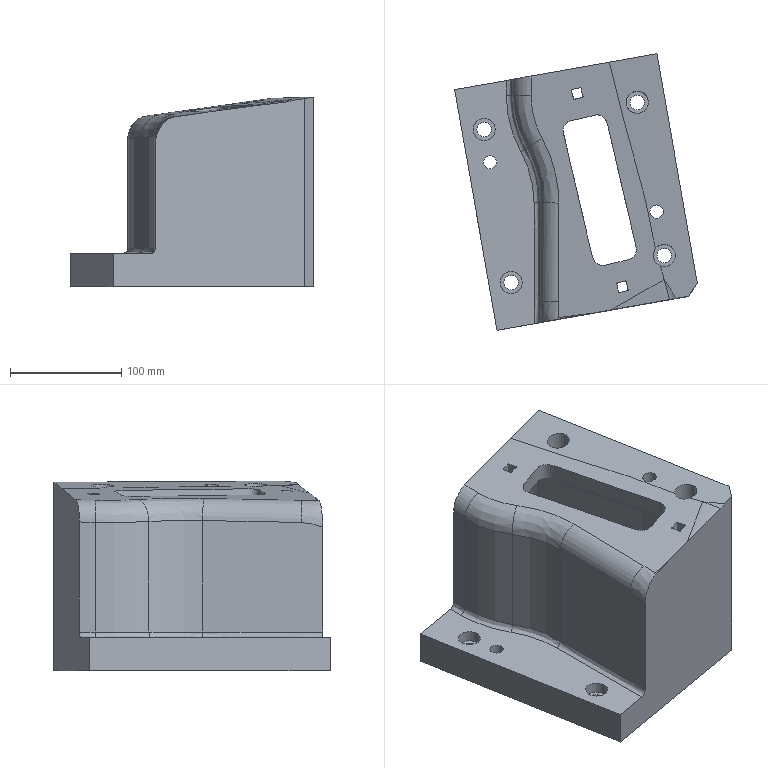Part | NX | features solid 2 | 1 solid | 49 faces | box 218.656 x 248.783 x 170.913 mm | volume 3486874 mm3 | spline 23 | plane 14 | cylinder 12 | commonest cylinder face diameters 13 x4 20 x4 12 x2 50 x2